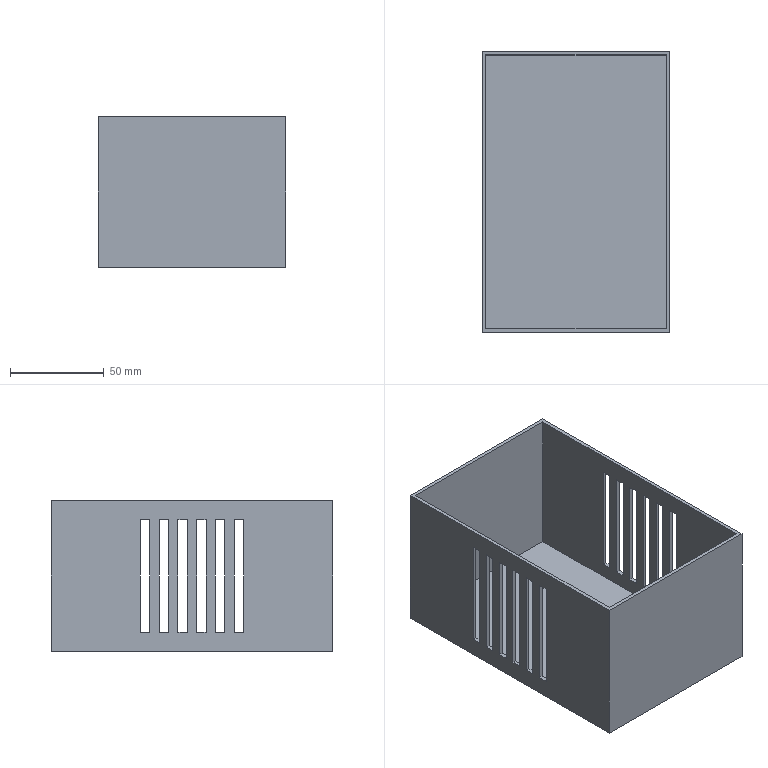Part | NX | 1 solid | 59 faces | box 100 x 150 x 80 mm | volume 99552 mm3 | plane 59